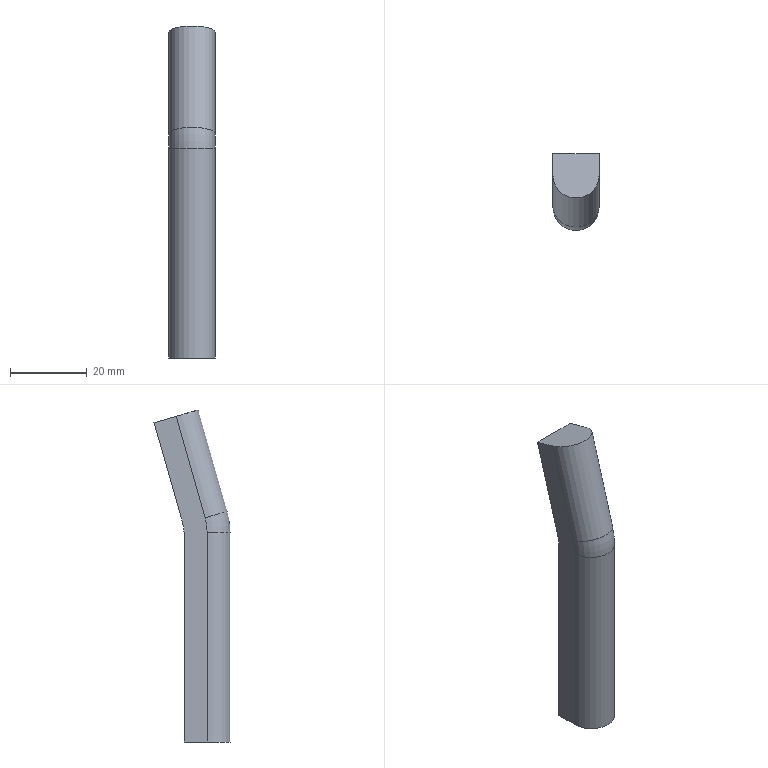Part | NX | features solid 2 | 1 solid | 10 faces | box 12 x 19.82 x 86.391 mm | volume 11015 mm3 | plane 6 | cylinder 3 | torus 1 | commonest cylinder face diameters 12 x2 16 x1
STEP:
#1=CARTESIAN_POINT('',(-423.,677.049,49.748));
#2=VERTEX_POINT('',#1);
#3=CARTESIAN_POINT('',(-435.,677.049,49.748));
#4=VERTEX_POINT('',#3);
#5=CARTESIAN_POINT('',(-429.,677.049,49.748));
#6=DIRECTION('',(0.,-0.2738,-0.9618));
#7=DIRECTION('',(0.,-0.9618,0.2738));
#8=AXIS2_PLACEMENT_3D('',#5,#6,#7);
#9=CIRCLE('',#8,6.);
#10=EDGE_CURVE('',#2,#4,#9,.T.);
#11=ORIENTED_EDGE('',*,*,#10,.F.);
#12=CARTESIAN_POINT('',(-423.,682.82,48.105));
#13=VERTEX_POINT('',#12);
#14=CARTESIAN_POINT('',(-423.,669.591,51.871));
#15=DIRECTION('',(0.,0.9618,-0.2738));
#16=VECTOR('',#15,1000.);
#17=LINE('',#14,#16);
#18=EDGE_CURVE('',#2,#13,#17,.T.);
#19=ORIENTED_EDGE('',*,*,#18,.T.);
#20=CARTESIAN_POINT('',(-435.,682.82,48.105));
#21=VERTEX_POINT('',#20);
#22=CARTESIAN_POINT('',(-379.25,682.82,48.105));
#23=DIRECTION('',(1.,0.,0.));
#24=VECTOR('',#23,1000.);
#25=LINE('',#22,#24);
#26=EDGE_CURVE('',#21,#13,#25,.T.);
#27=ORIENTED_EDGE('',*,*,#26,.F.);
#28=CARTESIAN_POINT('',(-435.,669.591,51.871));
#29=DIRECTION('',(0.,0.9618,-0.2738));
#30=VECTOR('',#29,1000.);
#31=LINE('',#28,#30);
#32=EDGE_CURVE('',#4,#21,#31,.T.);
#33=ORIENTED_EDGE('',*,*,#32,.F.);
#34=EDGE_LOOP('',(#11,#19,#27,#33));
#35=FACE_BOUND('',#34,.T.);
#36=CARTESIAN_POINT('',(-379.25,681.179,48.572));
#37=DIRECTION('',(0.,0.2738,0.9618));
#38=DIRECTION('',(0.,-0.9618,0.2738));
#39=AXIS2_PLACEMENT_3D('',#36,#37,#38);
#40=PLANE('',#39);
#41=ADVANCED_FACE('',(#35),#40,.T.);
#42=ORIENTED_EDGE('',*,*,#10,.T.);
#43=CARTESIAN_POINT('',(-435.,669.535,23.357));
#44=VERTEX_POINT('',#43);
#45=CARTESIAN_POINT('',(-435.,669.535,23.357));
#46=DIRECTION('',(0.,0.2738,0.9618));
#47=VECTOR('',#46,1000.);
#48=LINE('',#45,#47);
#49=EDGE_CURVE('',#44,#4,#48,.T.);
#50=ORIENTED_EDGE('',*,*,#49,.F.);
#51=CARTESIAN_POINT('',(-423.,669.535,23.357));
#52=VERTEX_POINT('',#51);
#53=CARTESIAN_POINT('',(-429.,669.535,23.357));
#54=DIRECTION('',(0.,-0.2738,-0.9618));
#55=DIRECTION('',(0.,-0.9618,0.2738));
#56=AXIS2_PLACEMENT_3D('',#53,#54,#55);
#57=CIRCLE('',#56,6.);
#58=EDGE_CURVE('',#52,#44,#57,.T.);
#59=ORIENTED_EDGE('',*,*,#58,.F.);
#60=CARTESIAN_POINT('',(-423.,669.535,23.357));
#61=DIRECTION('',(0.,0.2738,0.9618));
#62=VECTOR('',#61,1000.);
#63=LINE('',#60,#62);
#64=EDGE_CURVE('',#52,#2,#63,.T.);
#65=ORIENTED_EDGE('',*,*,#64,.T.);
#66=EDGE_LOOP('',(#42,#50,#59,#65));
#67=FACE_BOUND('',#66,.T.);
#68=CARTESIAN_POINT('',(-429.,669.535,23.357));
#69=DIRECTION('',(0.,0.2738,0.9618));
#70=DIRECTION('',(0.,-0.9618,0.2738));
#71=AXIS2_PLACEMENT_3D('',#68,#69,#70);
#72=CYLINDRICAL_SURFACE('',#71,6.);
#73=ADVANCED_FACE('',(#67),#72,.T.);
#74=CARTESIAN_POINT('',(-435.,675.,19.523));
#75=VERTEX_POINT('',#74);
#76=CARTESIAN_POINT('',(-435.,675.,-35.));
#77=VERTEX_POINT('',#76);
#78=CARTESIAN_POINT('',(-435.,675.,54.523));
#79=DIRECTION('',(0.,0.,-1.));
#80=VECTOR('',#79,1000.);
#81=LINE('',#78,#80);
#82=EDGE_CURVE('',#75,#77,#81,.T.);
#83=ORIENTED_EDGE('',*,*,#82,.T.);
#84=CARTESIAN_POINT('',(-435.,669.,-35.));
#85=VERTEX_POINT('',#84);
#86=CARTESIAN_POINT('',(-435.,767.,-35.));
#87=DIRECTION('',(0.,1.,0.));
#88=VECTOR('',#87,1000.);
#89=LINE('',#86,#88);
#90=EDGE_CURVE('',#85,#77,#89,.T.);
#91=ORIENTED_EDGE('',*,*,#90,.F.);
#92=CARTESIAN_POINT('',(-435.,669.,19.523));
#93=VERTEX_POINT('',#92);
#94=CARTESIAN_POINT('',(-435.,669.,34.523));
#95=DIRECTION('',(0.,0.,-1.));
#96=VECTOR('',#95,1000.);
#97=LINE('',#94,#96);
#98=EDGE_CURVE('',#93,#85,#97,.T.);
#99=ORIENTED_EDGE('',*,*,#98,.F.);
#100=CARTESIAN_POINT('',(-435.,683.,19.523));
#101=DIRECTION('',(-1.,0.,0.));
#102=DIRECTION('',(0.,0.,-1.));
#103=AXIS2_PLACEMENT_3D('',#100,#101,#102);
#104=CIRCLE('',#103,14.);
#105=EDGE_CURVE('',#93,#44,#104,.T.);
#106=ORIENTED_EDGE('',*,*,#105,.T.);
#107=ORIENTED_EDGE('',*,*,#49,.T.);
#108=ORIENTED_EDGE('',*,*,#32,.T.);
#109=CARTESIAN_POINT('',(-435.,675.306,21.714));
#110=VERTEX_POINT('',#109);
#111=CARTESIAN_POINT('',(-435.,675.306,21.714));
#112=DIRECTION('',(0.,0.2738,0.9618));
#113=VECTOR('',#112,1000.);
#114=LINE('',#111,#113);
#115=EDGE_CURVE('',#110,#21,#114,.T.);
#116=ORIENTED_EDGE('',*,*,#115,.F.);
#117=CARTESIAN_POINT('',(-435.,683.,19.523));
#118=DIRECTION('',(-1.,0.,0.));
#119=DIRECTION('',(0.,0.,-1.));
#120=AXIS2_PLACEMENT_3D('',#117,#118,#119);
#121=CIRCLE('',#120,8.);
#122=EDGE_CURVE('',#75,#110,#121,.T.);
#123=ORIENTED_EDGE('',*,*,#122,.F.);
#124=EDGE_LOOP('',(#83,#91,#99,#106,#107,#108,#116,#123));
#125=FACE_BOUND('',#124,.T.);
#126=CARTESIAN_POINT('',(-435.,842.,24.523));
#127=DIRECTION('',(1.,0.,0.));
#128=DIRECTION('',(0.,-1.,0.));
#129=AXIS2_PLACEMENT_3D('',#126,#127,#128);
#130=PLANE('',#129);
#131=ADVANCED_FACE('',(#125),#130,.F.);
#132=ORIENTED_EDGE('',*,*,#64,.F.);
#133=CARTESIAN_POINT('',(-423.,669.,19.523));
#134=VERTEX_POINT('',#133);
#135=CARTESIAN_POINT('',(-423.,683.,19.523));
#136=DIRECTION('',(-1.,0.,0.));
#137=DIRECTION('',(0.,0.,-1.));
#138=AXIS2_PLACEMENT_3D('',#135,#136,#137);
#139=CIRCLE('',#138,14.);
#140=EDGE_CURVE('',#134,#52,#139,.T.);
#141=ORIENTED_EDGE('',*,*,#140,.F.);
#142=CARTESIAN_POINT('',(-423.,669.,-35.));
#143=VERTEX_POINT('',#142);
#144=CARTESIAN_POINT('',(-423.,669.,34.523));
#145=DIRECTION('',(0.,0.,-1.));
#146=VECTOR('',#145,1000.);
#147=LINE('',#144,#146);
#148=EDGE_CURVE('',#134,#143,#147,.T.);
#149=ORIENTED_EDGE('',*,*,#148,.T.);
#150=CARTESIAN_POINT('',(-423.,675.,-35.));
#151=VERTEX_POINT('',#150);
#152=CARTESIAN_POINT('',(-423.,767.,-35.));
#153=DIRECTION('',(0.,-1.,0.));
#154=VECTOR('',#153,1000.);
#155=LINE('',#152,#154);
#156=EDGE_CURVE('',#151,#143,#155,.T.);
#157=ORIENTED_EDGE('',*,*,#156,.F.);
#158=CARTESIAN_POINT('',(-423.,675.,19.523));
#159=VERTEX_POINT('',#158);
#160=CARTESIAN_POINT('',(-423.,675.,54.523));
#161=DIRECTION('',(0.,0.,-1.));
#162=VECTOR('',#161,1000.);
#163=LINE('',#160,#162);
#164=EDGE_CURVE('',#159,#151,#163,.T.);
#165=ORIENTED_EDGE('',*,*,#164,.F.);
#166=CARTESIAN_POINT('',(-423.,675.306,21.714));
#167=VERTEX_POINT('',#166);
#168=CARTESIAN_POINT('',(-423.,683.,19.523));
#169=DIRECTION('',(-1.,0.,0.));
#170=DIRECTION('',(0.,0.,-1.));
#171=AXIS2_PLACEMENT_3D('',#168,#169,#170);
#172=CIRCLE('',#171,8.);
#173=EDGE_CURVE('',#159,#167,#172,.T.);
#174=ORIENTED_EDGE('',*,*,#173,.T.);
#175=CARTESIAN_POINT('',(-423.,675.306,21.714));
#176=DIRECTION('',(0.,0.2738,0.9618));
#177=VECTOR('',#176,1000.);
#178=LINE('',#175,#177);
#179=EDGE_CURVE('',#167,#13,#178,.T.);
#180=ORIENTED_EDGE('',*,*,#179,.T.);
#181=ORIENTED_EDGE('',*,*,#18,.F.);
#182=EDGE_LOOP('',(#132,#141,#149,#157,#165,#174,#180,#181));
#183=FACE_BOUND('',#182,.T.);
#184=CARTESIAN_POINT('',(-423.,736.,-65.));
#185=DIRECTION('',(-1.,0.,0.));
#186=DIRECTION('',(0.,0.,1.));
#187=AXIS2_PLACEMENT_3D('',#184,#185,#186);
#188=PLANE('',#187);
#189=ADVANCED_FACE('',(#183),#188,.F.);
#190=CARTESIAN_POINT('',(-228.,675.,-35.));
#191=DIRECTION('',(1.,0.,0.));
#192=VECTOR('',#191,1000.);
#193=LINE('',#190,#192);
#194=EDGE_CURVE('',#77,#151,#193,.T.);
#195=ORIENTED_EDGE('',*,*,#194,.T.);
#196=ORIENTED_EDGE('',*,*,#156,.T.);
#197=CARTESIAN_POINT('',(-429.,669.,-35.));
#198=DIRECTION('',(0.,0.,1.));
#199=DIRECTION('',(1.,0.,0.));
#200=AXIS2_PLACEMENT_3D('',#197,#198,#199);
#201=CIRCLE('',#200,6.);
#202=EDGE_CURVE('',#143,#85,#201,.F.);
#203=ORIENTED_EDGE('',*,*,#202,.T.);
#204=ORIENTED_EDGE('',*,*,#90,.T.);
#205=EDGE_LOOP('',(#195,#196,#203,#204));
#206=FACE_BOUND('',#205,.T.);
#207=CARTESIAN_POINT('',(-228.,767.,-35.));
#208=DIRECTION('',(0.,0.,1.));
#209=DIRECTION('',(0.,1.,0.));
#210=AXIS2_PLACEMENT_3D('',#207,#208,#209);
#211=PLANE('',#210);
#212=ADVANCED_FACE('',(#206),#211,.F.);
#213=ORIENTED_EDGE('',*,*,#164,.T.);
#214=ORIENTED_EDGE('',*,*,#194,.F.);
#215=ORIENTED_EDGE('',*,*,#82,.F.);
#216=CARTESIAN_POINT('',(-409.,675.,19.523));
#217=DIRECTION('',(1.,0.,0.));
#218=VECTOR('',#217,1000.);
#219=LINE('',#216,#218);
#220=EDGE_CURVE('',#75,#159,#219,.T.);
#221=ORIENTED_EDGE('',*,*,#220,.T.);
#222=EDGE_LOOP('',(#213,#214,#215,#221));
#223=FACE_BOUND('',#222,.T.);
#224=CARTESIAN_POINT('',(-409.,675.,54.523));
#225=DIRECTION('',(0.,-1.,0.));
#226=DIRECTION('',(-1.,0.,0.));
#227=AXIS2_PLACEMENT_3D('',#224,#225,#226);
#228=PLANE('',#227);
#229=ADVANCED_FACE('',(#223),#228,.F.);
#230=CARTESIAN_POINT('',(-429.,669.,19.523));
#231=DIRECTION('',(0.,0.,-1.));
#232=DIRECTION('',(0.,-1.,0.));
#233=AXIS2_PLACEMENT_3D('',#230,#231,#232);
#234=CIRCLE('',#233,6.);
#235=EDGE_CURVE('',#134,#93,#234,.T.);
#236=ORIENTED_EDGE('',*,*,#235,.F.);
#237=ORIENTED_EDGE('',*,*,#140,.T.);
#238=ORIENTED_EDGE('',*,*,#58,.T.);
#239=ORIENTED_EDGE('',*,*,#105,.F.);
#240=EDGE_LOOP('',(#236,#237,#238,#239));
#241=FACE_BOUND('',#240,.T.);
#242=CARTESIAN_POINT('',(-429.,683.,19.523));
#243=DIRECTION('',(1.,0.,0.));
#244=DIRECTION('',(0.,0.,-1.));
#245=AXIS2_PLACEMENT_3D('',#242,#243,#244);
#246=TOROIDAL_SURFACE('',#245,14.,6.);
#247=ADVANCED_FACE('',(#241),#246,.T.);
#248=ORIENTED_EDGE('',*,*,#98,.T.);
#249=ORIENTED_EDGE('',*,*,#202,.F.);
#250=ORIENTED_EDGE('',*,*,#148,.F.);
#251=ORIENTED_EDGE('',*,*,#235,.T.);
#252=EDGE_LOOP('',(#248,#249,#250,#251));
#253=FACE_BOUND('',#252,.T.);
#254=CARTESIAN_POINT('',(-429.,669.,34.523));
#255=DIRECTION('',(0.,0.,-1.));
#256=DIRECTION('',(0.,1.,0.));
#257=AXIS2_PLACEMENT_3D('',#254,#255,#256);
#258=CYLINDRICAL_SURFACE('',#257,6.);
#259=ADVANCED_FACE('',(#253),#258,.T.);
#260=CARTESIAN_POINT('',(-409.,675.306,21.714));
#261=DIRECTION('',(1.,0.,0.));
#262=VECTOR('',#261,1000.);
#263=LINE('',#260,#262);
#264=EDGE_CURVE('',#110,#167,#263,.T.);
#265=ORIENTED_EDGE('',*,*,#264,.F.);
#266=ORIENTED_EDGE('',*,*,#115,.T.);
#267=ORIENTED_EDGE('',*,*,#26,.T.);
#268=ORIENTED_EDGE('',*,*,#179,.F.);
#269=EDGE_LOOP('',(#265,#266,#267,#268));
#270=FACE_BOUND('',#269,.T.);
#271=CARTESIAN_POINT('',(-409.,675.306,21.714));
#272=DIRECTION('',(0.,0.9618,-0.2738));
#273=DIRECTION('',(0.,0.2738,0.9618));
#274=AXIS2_PLACEMENT_3D('',#271,#272,#273);
#275=PLANE('',#274);
#276=ADVANCED_FACE('',(#270),#275,.T.);
#277=ORIENTED_EDGE('',*,*,#220,.F.);
#278=ORIENTED_EDGE('',*,*,#122,.T.);
#279=ORIENTED_EDGE('',*,*,#264,.T.);
#280=ORIENTED_EDGE('',*,*,#173,.F.);
#281=EDGE_LOOP('',(#277,#278,#279,#280));
#282=FACE_BOUND('',#281,.T.);
#283=CARTESIAN_POINT('',(-394.,683.,19.523));
#284=DIRECTION('',(1.,0.,0.));
#285=DIRECTION('',(0.,0.,-1.));
#286=AXIS2_PLACEMENT_3D('',#283,#284,#285);
#287=CYLINDRICAL_SURFACE('',#286,8.);
#288=ADVANCED_FACE('',(#282),#287,.F.);
#289=CLOSED_SHELL('',(#41,#73,#131,#189,#212,#229,#247,#259,#276,#288));
#290=MANIFOLD_SOLID_BREP('',#289);
#291=(LENGTH_UNIT()NAMED_UNIT(*)SI_UNIT(.MILLI.,.METRE.));
#292=UNCERTAINTY_MEASURE_WITH_UNIT(LENGTH_MEASURE(0.00001),#291,'','');
#293=(NAMED_UNIT(*)PLANE_ANGLE_UNIT()SI_UNIT($,.RADIAN.));
#294=(NAMED_UNIT(*)SI_UNIT($,.STERADIAN.)SOLID_ANGLE_UNIT());
#295=(GEOMETRIC_REPRESENTATION_CONTEXT(3)GLOBAL_UNCERTAINTY_ASSIGNED_CONTEXT((#292))GLOBAL_UNIT_ASSIGNED_CONTEXT((#291,#293,#294))REPRESENTATION_CONTEXT('',''));
#296=ADVANCED_BREP_SHAPE_REPRESENTATION('',(#290),#295);